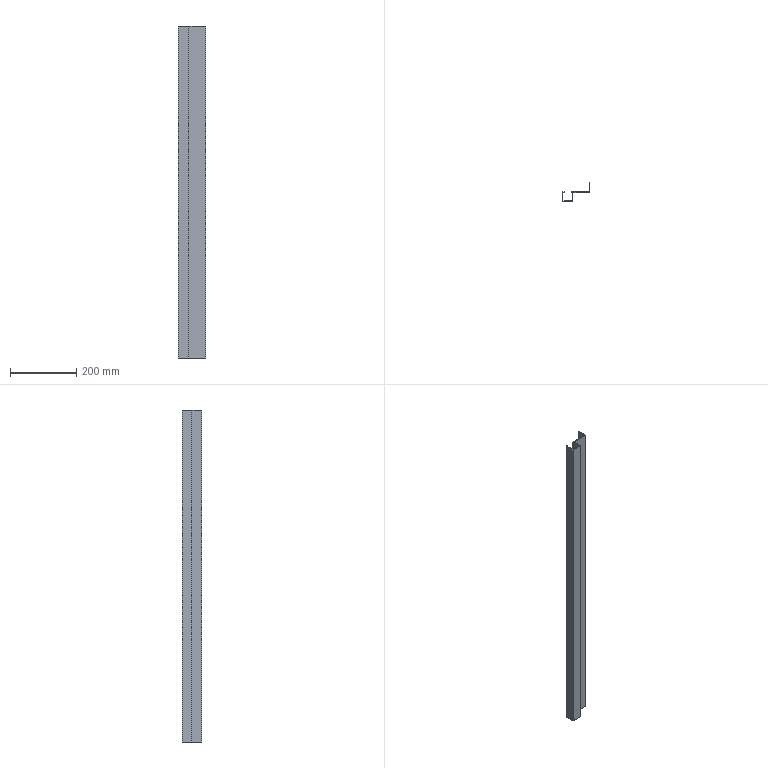Part | STEP file | Rieles_2-22 | 1 solid | 18 faces | box 81.4 x 57.7 x 999 mm | volume 260289 mm3 | plane 18
STEP:
#1=CARTESIAN_POINT('',(10.,26.2,-551.));
#2=VERTEX_POINT('',#1);
#3=CARTESIAN_POINT('',(10.,27.7,-551.));
#4=VERTEX_POINT('',#3);
#5=CARTESIAN_POINT('',(10.,27.35,-551.));
#6=DIRECTION('',(0.,1.,0.));
#7=VECTOR('',#6,1000.);
#8=LINE('',#5,#7);
#9=EDGE_CURVE('',#2,#4,#8,.T.);
#10=ORIENTED_EDGE('',*,*,#9,.T.);
#11=CARTESIAN_POINT('',(64.2,27.7,-551.));
#12=VERTEX_POINT('',#11);
#13=CARTESIAN_POINT('',(25.,27.7,-551.));
#14=DIRECTION('',(1.,0.,0.));
#15=VECTOR('',#14,1000.);
#16=LINE('',#13,#15);
#17=EDGE_CURVE('',#4,#12,#16,.T.);
#18=ORIENTED_EDGE('',*,*,#17,.T.);
#19=CARTESIAN_POINT('',(64.2,56.2,-551.));
#20=VERTEX_POINT('',#19);
#21=CARTESIAN_POINT('',(64.2,27.35,-551.));
#22=DIRECTION('',(0.,1.,0.));
#23=VECTOR('',#22,1000.);
#24=LINE('',#21,#23);
#25=EDGE_CURVE('',#12,#20,#24,.T.);
#26=ORIENTED_EDGE('',*,*,#25,.T.);
#27=CARTESIAN_POINT('',(65.7,56.2,-551.));
#28=VERTEX_POINT('',#27);
#29=CARTESIAN_POINT('',(25.,56.2,-551.));
#30=DIRECTION('',(1.,0.,0.));
#31=VECTOR('',#30,1000.);
#32=LINE('',#29,#31);
#33=EDGE_CURVE('',#20,#28,#32,.T.);
#34=ORIENTED_EDGE('',*,*,#33,.T.);
#35=CARTESIAN_POINT('',(65.7,26.2,-551.));
#36=VERTEX_POINT('',#35);
#37=CARTESIAN_POINT('',(65.7,27.35,-551.));
#38=DIRECTION('',(0.,-1.,0.));
#39=VECTOR('',#38,1000.);
#40=LINE('',#37,#39);
#41=EDGE_CURVE('',#28,#36,#40,.T.);
#42=ORIENTED_EDGE('',*,*,#41,.T.);
#43=CARTESIAN_POINT('',(15.7,26.2,-551.));
#44=VERTEX_POINT('',#43);
#45=CARTESIAN_POINT('',(25.,26.2,-551.));
#46=DIRECTION('',(-1.,0.,0.));
#47=VECTOR('',#46,1000.);
#48=LINE('',#45,#47);
#49=EDGE_CURVE('',#36,#44,#48,.T.);
#50=ORIENTED_EDGE('',*,*,#49,.T.);
#51=CARTESIAN_POINT('',(15.7,-1.5,-551.));
#52=VERTEX_POINT('',#51);
#53=CARTESIAN_POINT('',(15.7,27.35,-551.));
#54=DIRECTION('',(0.,-1.,0.));
#55=VECTOR('',#54,1000.);
#56=LINE('',#53,#55);
#57=EDGE_CURVE('',#44,#52,#56,.T.);
#58=ORIENTED_EDGE('',*,*,#57,.T.);
#59=CARTESIAN_POINT('',(-15.7,-1.5,-551.));
#60=VERTEX_POINT('',#59);
#61=CARTESIAN_POINT('',(25.,-1.5,-551.));
#62=DIRECTION('',(-1.,0.,0.));
#63=VECTOR('',#62,1000.);
#64=LINE('',#61,#63);
#65=EDGE_CURVE('',#52,#60,#64,.T.);
#66=ORIENTED_EDGE('',*,*,#65,.T.);
#67=CARTESIAN_POINT('',(-15.7,27.7,-551.));
#68=VERTEX_POINT('',#67);
#69=CARTESIAN_POINT('',(-15.7,27.35,-551.));
#70=DIRECTION('',(0.,1.,0.));
#71=VECTOR('',#70,1000.);
#72=LINE('',#69,#71);
#73=EDGE_CURVE('',#60,#68,#72,.T.);
#74=ORIENTED_EDGE('',*,*,#73,.T.);
#75=CARTESIAN_POINT('',(-10.,27.7,-551.));
#76=VERTEX_POINT('',#75);
#77=CARTESIAN_POINT('',(25.,27.7,-551.));
#78=DIRECTION('',(1.,0.,0.));
#79=VECTOR('',#78,1000.);
#80=LINE('',#77,#79);
#81=EDGE_CURVE('',#68,#76,#80,.T.);
#82=ORIENTED_EDGE('',*,*,#81,.T.);
#83=CARTESIAN_POINT('',(-10.,26.2,-551.));
#84=VERTEX_POINT('',#83);
#85=CARTESIAN_POINT('',(-10.,27.35,-551.));
#86=DIRECTION('',(0.,-1.,0.));
#87=VECTOR('',#86,1000.);
#88=LINE('',#85,#87);
#89=EDGE_CURVE('',#76,#84,#88,.T.);
#90=ORIENTED_EDGE('',*,*,#89,.T.);
#91=CARTESIAN_POINT('',(-14.2,26.2,-551.));
#92=VERTEX_POINT('',#91);
#93=CARTESIAN_POINT('',(25.,26.2,-551.));
#94=DIRECTION('',(-1.,0.,0.));
#95=VECTOR('',#94,1000.);
#96=LINE('',#93,#95);
#97=EDGE_CURVE('',#84,#92,#96,.T.);
#98=ORIENTED_EDGE('',*,*,#97,.T.);
#99=CARTESIAN_POINT('',(-14.2,0.,-551.));
#100=VERTEX_POINT('',#99);
#101=CARTESIAN_POINT('',(-14.2,27.35,-551.));
#102=DIRECTION('',(0.,-1.,0.));
#103=VECTOR('',#102,1000.);
#104=LINE('',#101,#103);
#105=EDGE_CURVE('',#92,#100,#104,.T.);
#106=ORIENTED_EDGE('',*,*,#105,.T.);
#107=CARTESIAN_POINT('',(14.2,0.,-551.));
#108=VERTEX_POINT('',#107);
#109=CARTESIAN_POINT('',(25.,0.,-551.));
#110=DIRECTION('',(1.,0.,0.));
#111=VECTOR('',#110,1000.);
#112=LINE('',#109,#111);
#113=EDGE_CURVE('',#100,#108,#112,.T.);
#114=ORIENTED_EDGE('',*,*,#113,.T.);
#115=CARTESIAN_POINT('',(14.2,26.2,-551.));
#116=VERTEX_POINT('',#115);
#117=CARTESIAN_POINT('',(14.2,27.35,-551.));
#118=DIRECTION('',(0.,1.,0.));
#119=VECTOR('',#118,1000.);
#120=LINE('',#117,#119);
#121=EDGE_CURVE('',#108,#116,#120,.T.);
#122=ORIENTED_EDGE('',*,*,#121,.T.);
#123=CARTESIAN_POINT('',(25.,26.2,-551.));
#124=DIRECTION('',(-1.,0.,0.));
#125=VECTOR('',#124,1000.);
#126=LINE('',#123,#125);
#127=EDGE_CURVE('',#116,#2,#126,.T.);
#128=ORIENTED_EDGE('',*,*,#127,.T.);
#129=EDGE_LOOP('',(#10,#18,#26,#34,#42,#50,#58,#66,#74,#82,#90,#98,#106,#114,#122,#128));
#130=FACE_OUTER_BOUND('',#129,.T.);
#131=CARTESIAN_POINT('',(25.,27.35,-551.));
#132=DIRECTION('',(0.,0.,-1.));
#133=DIRECTION('',(0.,-1.,0.));
#134=AXIS2_PLACEMENT_3D('',#131,#132,#133);
#135=PLANE('',#134);
#136=ADVANCED_FACE('',(#130),#135,.T.);
#137=CARTESIAN_POINT('',(10.,26.2,448.));
#138=VERTEX_POINT('',#137);
#139=CARTESIAN_POINT('',(10.,27.7,448.));
#140=VERTEX_POINT('',#139);
#141=CARTESIAN_POINT('',(10.,26.2,448.));
#142=DIRECTION('',(0.,1.,0.));
#143=VECTOR('',#142,1000.);
#144=LINE('',#141,#143);
#145=EDGE_CURVE('',#138,#140,#144,.T.);
#146=ORIENTED_EDGE('',*,*,#145,.F.);
#147=CARTESIAN_POINT('',(14.2,26.2,448.));
#148=VERTEX_POINT('',#147);
#149=CARTESIAN_POINT('',(14.2,26.2,448.));
#150=DIRECTION('',(-1.,0.,0.));
#151=VECTOR('',#150,1000.);
#152=LINE('',#149,#151);
#153=EDGE_CURVE('',#148,#138,#152,.T.);
#154=ORIENTED_EDGE('',*,*,#153,.F.);
#155=CARTESIAN_POINT('',(14.2,0.,448.));
#156=VERTEX_POINT('',#155);
#157=CARTESIAN_POINT('',(14.2,0.,448.));
#158=DIRECTION('',(0.,1.,0.));
#159=VECTOR('',#158,1000.);
#160=LINE('',#157,#159);
#161=EDGE_CURVE('',#156,#148,#160,.T.);
#162=ORIENTED_EDGE('',*,*,#161,.F.);
#163=CARTESIAN_POINT('',(-14.2,0.,448.));
#164=VERTEX_POINT('',#163);
#165=CARTESIAN_POINT('',(-14.2,0.,448.));
#166=DIRECTION('',(1.,0.,0.));
#167=VECTOR('',#166,1000.);
#168=LINE('',#165,#167);
#169=EDGE_CURVE('',#164,#156,#168,.T.);
#170=ORIENTED_EDGE('',*,*,#169,.F.);
#171=CARTESIAN_POINT('',(-14.2,26.2,448.));
#172=VERTEX_POINT('',#171);
#173=CARTESIAN_POINT('',(-14.2,26.2,448.));
#174=DIRECTION('',(0.,-1.,0.));
#175=VECTOR('',#174,1000.);
#176=LINE('',#173,#175);
#177=EDGE_CURVE('',#172,#164,#176,.T.);
#178=ORIENTED_EDGE('',*,*,#177,.F.);
#179=CARTESIAN_POINT('',(-10.,26.2,448.));
#180=VERTEX_POINT('',#179);
#181=CARTESIAN_POINT('',(-10.,26.2,448.));
#182=DIRECTION('',(-1.,0.,0.));
#183=VECTOR('',#182,1000.);
#184=LINE('',#181,#183);
#185=EDGE_CURVE('',#180,#172,#184,.T.);
#186=ORIENTED_EDGE('',*,*,#185,.F.);
#187=CARTESIAN_POINT('',(-10.,27.7,448.));
#188=VERTEX_POINT('',#187);
#189=CARTESIAN_POINT('',(-10.,27.7,448.));
#190=DIRECTION('',(0.,-1.,0.));
#191=VECTOR('',#190,1000.);
#192=LINE('',#189,#191);
#193=EDGE_CURVE('',#188,#180,#192,.T.);
#194=ORIENTED_EDGE('',*,*,#193,.F.);
#195=CARTESIAN_POINT('',(-15.7,27.7,448.));
#196=VERTEX_POINT('',#195);
#197=CARTESIAN_POINT('',(-15.7,27.7,448.));
#198=DIRECTION('',(1.,0.,0.));
#199=VECTOR('',#198,1000.);
#200=LINE('',#197,#199);
#201=EDGE_CURVE('',#196,#188,#200,.T.);
#202=ORIENTED_EDGE('',*,*,#201,.F.);
#203=CARTESIAN_POINT('',(-15.7,-1.5,448.));
#204=VERTEX_POINT('',#203);
#205=CARTESIAN_POINT('',(-15.7,-1.5,448.));
#206=DIRECTION('',(0.,1.,0.));
#207=VECTOR('',#206,1000.);
#208=LINE('',#205,#207);
#209=EDGE_CURVE('',#204,#196,#208,.T.);
#210=ORIENTED_EDGE('',*,*,#209,.F.);
#211=CARTESIAN_POINT('',(15.7,-1.5,448.));
#212=VERTEX_POINT('',#211);
#213=CARTESIAN_POINT('',(15.7,-1.5,448.));
#214=DIRECTION('',(-1.,0.,0.));
#215=VECTOR('',#214,1000.);
#216=LINE('',#213,#215);
#217=EDGE_CURVE('',#212,#204,#216,.T.);
#218=ORIENTED_EDGE('',*,*,#217,.F.);
#219=CARTESIAN_POINT('',(15.7,26.2,448.));
#220=VERTEX_POINT('',#219);
#221=CARTESIAN_POINT('',(15.7,26.2,448.));
#222=DIRECTION('',(0.,-1.,0.));
#223=VECTOR('',#222,1000.);
#224=LINE('',#221,#223);
#225=EDGE_CURVE('',#220,#212,#224,.T.);
#226=ORIENTED_EDGE('',*,*,#225,.F.);
#227=CARTESIAN_POINT('',(65.7,26.2,448.));
#228=VERTEX_POINT('',#227);
#229=CARTESIAN_POINT('',(65.7,26.2,448.));
#230=DIRECTION('',(-1.,0.,0.));
#231=VECTOR('',#230,1000.);
#232=LINE('',#229,#231);
#233=EDGE_CURVE('',#228,#220,#232,.T.);
#234=ORIENTED_EDGE('',*,*,#233,.F.);
#235=CARTESIAN_POINT('',(65.7,56.2,448.));
#236=VERTEX_POINT('',#235);
#237=CARTESIAN_POINT('',(65.7,56.2,448.));
#238=DIRECTION('',(0.,-1.,0.));
#239=VECTOR('',#238,1000.);
#240=LINE('',#237,#239);
#241=EDGE_CURVE('',#236,#228,#240,.T.);
#242=ORIENTED_EDGE('',*,*,#241,.F.);
#243=CARTESIAN_POINT('',(64.2,56.2,448.));
#244=VERTEX_POINT('',#243);
#245=CARTESIAN_POINT('',(64.2,56.2,448.));
#246=DIRECTION('',(1.,0.,0.));
#247=VECTOR('',#246,1000.);
#248=LINE('',#245,#247);
#249=EDGE_CURVE('',#244,#236,#248,.T.);
#250=ORIENTED_EDGE('',*,*,#249,.F.);
#251=CARTESIAN_POINT('',(64.2,27.7,448.));
#252=VERTEX_POINT('',#251);
#253=CARTESIAN_POINT('',(64.2,27.7,448.));
#254=DIRECTION('',(0.,1.,0.));
#255=VECTOR('',#254,1000.);
#256=LINE('',#253,#255);
#257=EDGE_CURVE('',#252,#244,#256,.T.);
#258=ORIENTED_EDGE('',*,*,#257,.F.);
#259=CARTESIAN_POINT('',(10.,27.7,448.));
#260=DIRECTION('',(1.,0.,0.));
#261=VECTOR('',#260,1000.);
#262=LINE('',#259,#261);
#263=EDGE_CURVE('',#140,#252,#262,.T.);
#264=ORIENTED_EDGE('',*,*,#263,.F.);
#265=EDGE_LOOP('',(#146,#154,#162,#170,#178,#186,#194,#202,#210,#218,#226,#234,#242,#250,#258,#264));
#266=FACE_OUTER_BOUND('',#265,.T.);
#267=CARTESIAN_POINT('',(25.,27.35,448.));
#268=DIRECTION('',(0.,0.,1.));
#269=DIRECTION('',(1.,0.,0.));
#270=AXIS2_PLACEMENT_3D('',#267,#268,#269);
#271=PLANE('',#270);
#272=ADVANCED_FACE('',(#266),#271,.T.);
#273=ORIENTED_EDGE('',*,*,#145,.T.);
#274=CARTESIAN_POINT('',(10.,27.7,407.));
#275=DIRECTION('',(0.,0.,-1.));
#276=VECTOR('',#275,1000.);
#277=LINE('',#274,#276);
#278=EDGE_CURVE('',#140,#4,#277,.T.);
#279=ORIENTED_EDGE('',*,*,#278,.T.);
#280=ORIENTED_EDGE('',*,*,#9,.F.);
#281=CARTESIAN_POINT('',(10.,26.2,407.));
#282=DIRECTION('',(0.,0.,-1.));
#283=VECTOR('',#282,1000.);
#284=LINE('',#281,#283);
#285=EDGE_CURVE('',#138,#2,#284,.T.);
#286=ORIENTED_EDGE('',*,*,#285,.F.);
#287=EDGE_LOOP('',(#273,#279,#280,#286));
#288=FACE_OUTER_BOUND('',#287,.T.);
#289=CARTESIAN_POINT('',(10.,26.2,407.));
#290=DIRECTION('',(-1.,0.,0.));
#291=DIRECTION('',(0.,0.,1.));
#292=AXIS2_PLACEMENT_3D('',#289,#290,#291);
#293=PLANE('',#292);
#294=ADVANCED_FACE('',(#288),#293,.T.);
#295=ORIENTED_EDGE('',*,*,#263,.T.);
#296=CARTESIAN_POINT('',(64.2,27.7,407.));
#297=DIRECTION('',(0.,0.,-1.));
#298=VECTOR('',#297,1000.);
#299=LINE('',#296,#298);
#300=EDGE_CURVE('',#252,#12,#299,.T.);
#301=ORIENTED_EDGE('',*,*,#300,.T.);
#302=ORIENTED_EDGE('',*,*,#17,.F.);
#303=ORIENTED_EDGE('',*,*,#278,.F.);
#304=EDGE_LOOP('',(#295,#301,#302,#303));
#305=FACE_OUTER_BOUND('',#304,.T.);
#306=CARTESIAN_POINT('',(10.,27.7,407.));
#307=DIRECTION('',(0.,1.,0.));
#308=DIRECTION('',(1.,0.,0.));
#309=AXIS2_PLACEMENT_3D('',#306,#307,#308);
#310=PLANE('',#309);
#311=ADVANCED_FACE('',(#305),#310,.T.);
#312=ORIENTED_EDGE('',*,*,#257,.T.);
#313=CARTESIAN_POINT('',(64.2,56.2,407.));
#314=DIRECTION('',(0.,0.,-1.));
#315=VECTOR('',#314,1000.);
#316=LINE('',#313,#315);
#317=EDGE_CURVE('',#244,#20,#316,.T.);
#318=ORIENTED_EDGE('',*,*,#317,.T.);
#319=ORIENTED_EDGE('',*,*,#25,.F.);
#320=ORIENTED_EDGE('',*,*,#300,.F.);
#321=EDGE_LOOP('',(#312,#318,#319,#320));
#322=FACE_OUTER_BOUND('',#321,.T.);
#323=CARTESIAN_POINT('',(64.2,27.7,407.));
#324=DIRECTION('',(-1.,0.,0.));
#325=DIRECTION('',(0.,0.,1.));
#326=AXIS2_PLACEMENT_3D('',#323,#324,#325);
#327=PLANE('',#326);
#328=ADVANCED_FACE('',(#322),#327,.T.);
#329=ORIENTED_EDGE('',*,*,#249,.T.);
#330=CARTESIAN_POINT('',(65.7,56.2,407.));
#331=DIRECTION('',(0.,0.,-1.));
#332=VECTOR('',#331,1000.);
#333=LINE('',#330,#332);
#334=EDGE_CURVE('',#236,#28,#333,.T.);
#335=ORIENTED_EDGE('',*,*,#334,.T.);
#336=ORIENTED_EDGE('',*,*,#33,.F.);
#337=ORIENTED_EDGE('',*,*,#317,.F.);
#338=EDGE_LOOP('',(#329,#335,#336,#337));
#339=FACE_OUTER_BOUND('',#338,.T.);
#340=CARTESIAN_POINT('',(64.2,56.2,407.));
#341=DIRECTION('',(0.,1.,0.));
#342=DIRECTION('',(1.,0.,0.));
#343=AXIS2_PLACEMENT_3D('',#340,#341,#342);
#344=PLANE('',#343);
#345=ADVANCED_FACE('',(#339),#344,.T.);
#346=ORIENTED_EDGE('',*,*,#241,.T.);
#347=CARTESIAN_POINT('',(65.7,26.2,407.));
#348=DIRECTION('',(0.,0.,-1.));
#349=VECTOR('',#348,1000.);
#350=LINE('',#347,#349);
#351=EDGE_CURVE('',#228,#36,#350,.T.);
#352=ORIENTED_EDGE('',*,*,#351,.T.);
#353=ORIENTED_EDGE('',*,*,#41,.F.);
#354=ORIENTED_EDGE('',*,*,#334,.F.);
#355=EDGE_LOOP('',(#346,#352,#353,#354));
#356=FACE_OUTER_BOUND('',#355,.T.);
#357=CARTESIAN_POINT('',(65.7,56.2,407.));
#358=DIRECTION('',(1.,0.,0.));
#359=DIRECTION('',(0.,-1.,0.));
#360=AXIS2_PLACEMENT_3D('',#357,#358,#359);
#361=PLANE('',#360);
#362=ADVANCED_FACE('',(#356),#361,.T.);
#363=ORIENTED_EDGE('',*,*,#233,.T.);
#364=CARTESIAN_POINT('',(15.7,26.2,407.));
#365=DIRECTION('',(0.,0.,-1.));
#366=VECTOR('',#365,1000.);
#367=LINE('',#364,#366);
#368=EDGE_CURVE('',#220,#44,#367,.T.);
#369=ORIENTED_EDGE('',*,*,#368,.T.);
#370=ORIENTED_EDGE('',*,*,#49,.F.);
#371=ORIENTED_EDGE('',*,*,#351,.F.);
#372=EDGE_LOOP('',(#363,#369,#370,#371));
#373=FACE_OUTER_BOUND('',#372,.T.);
#374=CARTESIAN_POINT('',(65.7,26.2,407.));
#375=DIRECTION('',(0.,-1.,0.));
#376=DIRECTION('',(0.,0.,-1.));
#377=AXIS2_PLACEMENT_3D('',#374,#375,#376);
#378=PLANE('',#377);
#379=ADVANCED_FACE('',(#373),#378,.T.);
#380=ORIENTED_EDGE('',*,*,#225,.T.);
#381=CARTESIAN_POINT('',(15.7,-1.5,407.));
#382=DIRECTION('',(0.,0.,-1.));
#383=VECTOR('',#382,1000.);
#384=LINE('',#381,#383);
#385=EDGE_CURVE('',#212,#52,#384,.T.);
#386=ORIENTED_EDGE('',*,*,#385,.T.);
#387=ORIENTED_EDGE('',*,*,#57,.F.);
#388=ORIENTED_EDGE('',*,*,#368,.F.);
#389=EDGE_LOOP('',(#380,#386,#387,#388));
#390=FACE_OUTER_BOUND('',#389,.T.);
#391=CARTESIAN_POINT('',(15.7,26.2,407.));
#392=DIRECTION('',(1.,0.,0.));
#393=DIRECTION('',(0.,1.,0.));
#394=AXIS2_PLACEMENT_3D('',#391,#392,#393);
#395=PLANE('',#394);
#396=ADVANCED_FACE('',(#390),#395,.T.);
#397=ORIENTED_EDGE('',*,*,#217,.T.);
#398=CARTESIAN_POINT('',(-15.7,-1.5,407.));
#399=DIRECTION('',(0.,0.,-1.));
#400=VECTOR('',#399,1000.);
#401=LINE('',#398,#400);
#402=EDGE_CURVE('',#204,#60,#401,.T.);
#403=ORIENTED_EDGE('',*,*,#402,.T.);
#404=ORIENTED_EDGE('',*,*,#65,.F.);
#405=ORIENTED_EDGE('',*,*,#385,.F.);
#406=EDGE_LOOP('',(#397,#403,#404,#405));
#407=FACE_OUTER_BOUND('',#406,.T.);
#408=CARTESIAN_POINT('',(15.7,-1.5,407.));
#409=DIRECTION('',(0.,-1.,0.));
#410=DIRECTION('',(0.,0.,-1.));
#411=AXIS2_PLACEMENT_3D('',#408,#409,#410);
#412=PLANE('',#411);
#413=ADVANCED_FACE('',(#407),#412,.T.);
#414=ORIENTED_EDGE('',*,*,#209,.T.);
#415=CARTESIAN_POINT('',(-15.7,27.7,407.));
#416=DIRECTION('',(0.,0.,-1.));
#417=VECTOR('',#416,1000.);
#418=LINE('',#415,#417);
#419=EDGE_CURVE('',#196,#68,#418,.T.);
#420=ORIENTED_EDGE('',*,*,#419,.T.);
#421=ORIENTED_EDGE('',*,*,#73,.F.);
#422=ORIENTED_EDGE('',*,*,#402,.F.);
#423=EDGE_LOOP('',(#414,#420,#421,#422));
#424=FACE_OUTER_BOUND('',#423,.T.);
#425=CARTESIAN_POINT('',(-15.7,-1.5,407.));
#426=DIRECTION('',(-1.,0.,0.));
#427=DIRECTION('',(0.,0.,1.));
#428=AXIS2_PLACEMENT_3D('',#425,#426,#427);
#429=PLANE('',#428);
#430=ADVANCED_FACE('',(#424),#429,.T.);
#431=ORIENTED_EDGE('',*,*,#201,.T.);
#432=CARTESIAN_POINT('',(-10.,27.7,407.));
#433=DIRECTION('',(0.,0.,-1.));
#434=VECTOR('',#433,1000.);
#435=LINE('',#432,#434);
#436=EDGE_CURVE('',#188,#76,#435,.T.);
#437=ORIENTED_EDGE('',*,*,#436,.T.);
#438=ORIENTED_EDGE('',*,*,#81,.F.);
#439=ORIENTED_EDGE('',*,*,#419,.F.);
#440=EDGE_LOOP('',(#431,#437,#438,#439));
#441=FACE_OUTER_BOUND('',#440,.T.);
#442=CARTESIAN_POINT('',(-15.7,27.7,407.));
#443=DIRECTION('',(0.,1.,0.));
#444=DIRECTION('',(1.,0.,0.));
#445=AXIS2_PLACEMENT_3D('',#442,#443,#444);
#446=PLANE('',#445);
#447=ADVANCED_FACE('',(#441),#446,.T.);
#448=ORIENTED_EDGE('',*,*,#193,.T.);
#449=CARTESIAN_POINT('',(-10.,26.2,407.));
#450=DIRECTION('',(0.,0.,-1.));
#451=VECTOR('',#450,1000.);
#452=LINE('',#449,#451);
#453=EDGE_CURVE('',#180,#84,#452,.T.);
#454=ORIENTED_EDGE('',*,*,#453,.T.);
#455=ORIENTED_EDGE('',*,*,#89,.F.);
#456=ORIENTED_EDGE('',*,*,#436,.F.);
#457=EDGE_LOOP('',(#448,#454,#455,#456));
#458=FACE_OUTER_BOUND('',#457,.T.);
#459=CARTESIAN_POINT('',(-10.,27.7,407.));
#460=DIRECTION('',(1.,0.,0.));
#461=DIRECTION('',(0.,1.,0.));
#462=AXIS2_PLACEMENT_3D('',#459,#460,#461);
#463=PLANE('',#462);
#464=ADVANCED_FACE('',(#458),#463,.T.);
#465=ORIENTED_EDGE('',*,*,#185,.T.);
#466=CARTESIAN_POINT('',(-14.2,26.2,407.));
#467=DIRECTION('',(0.,0.,-1.));
#468=VECTOR('',#467,1000.);
#469=LINE('',#466,#468);
#470=EDGE_CURVE('',#172,#92,#469,.T.);
#471=ORIENTED_EDGE('',*,*,#470,.T.);
#472=ORIENTED_EDGE('',*,*,#97,.F.);
#473=ORIENTED_EDGE('',*,*,#453,.F.);
#474=EDGE_LOOP('',(#465,#471,#472,#473));
#475=FACE_OUTER_BOUND('',#474,.T.);
#476=CARTESIAN_POINT('',(-10.,26.2,407.));
#477=DIRECTION('',(0.,-1.,0.));
#478=DIRECTION('',(0.,0.,-1.));
#479=AXIS2_PLACEMENT_3D('',#476,#477,#478);
#480=PLANE('',#479);
#481=ADVANCED_FACE('',(#475),#480,.T.);
#482=ORIENTED_EDGE('',*,*,#177,.T.);
#483=CARTESIAN_POINT('',(-14.2,0.,407.));
#484=DIRECTION('',(0.,0.,-1.));
#485=VECTOR('',#484,1000.);
#486=LINE('',#483,#485);
#487=EDGE_CURVE('',#164,#100,#486,.T.);
#488=ORIENTED_EDGE('',*,*,#487,.T.);
#489=ORIENTED_EDGE('',*,*,#105,.F.);
#490=ORIENTED_EDGE('',*,*,#470,.F.);
#491=EDGE_LOOP('',(#482,#488,#489,#490));
#492=FACE_OUTER_BOUND('',#491,.T.);
#493=CARTESIAN_POINT('',(-14.2,26.2,407.));
#494=DIRECTION('',(1.,0.,0.));
#495=DIRECTION('',(0.,1.,0.));
#496=AXIS2_PLACEMENT_3D('',#493,#494,#495);
#497=PLANE('',#496);
#498=ADVANCED_FACE('',(#492),#497,.T.);
#499=ORIENTED_EDGE('',*,*,#169,.T.);
#500=CARTESIAN_POINT('',(14.2,0.,407.));
#501=DIRECTION('',(0.,0.,-1.));
#502=VECTOR('',#501,1000.);
#503=LINE('',#500,#502);
#504=EDGE_CURVE('',#156,#108,#503,.T.);
#505=ORIENTED_EDGE('',*,*,#504,.T.);
#506=ORIENTED_EDGE('',*,*,#113,.F.);
#507=ORIENTED_EDGE('',*,*,#487,.F.);
#508=EDGE_LOOP('',(#499,#505,#506,#507));
#509=FACE_OUTER_BOUND('',#508,.T.);
#510=CARTESIAN_POINT('',(-14.2,0.,407.));
#511=DIRECTION('',(0.,1.,0.));
#512=DIRECTION('',(1.,0.,0.));
#513=AXIS2_PLACEMENT_3D('',#510,#511,#512);
#514=PLANE('',#513);
#515=ADVANCED_FACE('',(#509),#514,.T.);
#516=ORIENTED_EDGE('',*,*,#161,.T.);
#517=CARTESIAN_POINT('',(14.2,26.2,407.));
#518=DIRECTION('',(0.,0.,-1.));
#519=VECTOR('',#518,1000.);
#520=LINE('',#517,#519);
#521=EDGE_CURVE('',#148,#116,#520,.T.);
#522=ORIENTED_EDGE('',*,*,#521,.T.);
#523=ORIENTED_EDGE('',*,*,#121,.F.);
#524=ORIENTED_EDGE('',*,*,#504,.F.);
#525=EDGE_LOOP('',(#516,#522,#523,#524));
#526=FACE_OUTER_BOUND('',#525,.T.);
#527=CARTESIAN_POINT('',(14.2,0.,407.));
#528=DIRECTION('',(-1.,0.,0.));
#529=DIRECTION('',(0.,0.,1.));
#530=AXIS2_PLACEMENT_3D('',#527,#528,#529);
#531=PLANE('',#530);
#532=ADVANCED_FACE('',(#526),#531,.T.);
#533=ORIENTED_EDGE('',*,*,#153,.T.);
#534=ORIENTED_EDGE('',*,*,#285,.T.);
#535=ORIENTED_EDGE('',*,*,#127,.F.);
#536=ORIENTED_EDGE('',*,*,#521,.F.);
#537=EDGE_LOOP('',(#533,#534,#535,#536));
#538=FACE_OUTER_BOUND('',#537,.T.);
#539=CARTESIAN_POINT('',(14.2,26.2,407.));
#540=DIRECTION('',(0.,-1.,0.));
#541=DIRECTION('',(-1.,0.,0.));
#542=AXIS2_PLACEMENT_3D('',#539,#540,#541);
#543=PLANE('',#542);
#544=ADVANCED_FACE('',(#538),#543,.T.);
#545=CLOSED_SHELL('',(#136,#272,#294,#311,#328,#345,#362,#379,#396,#413,#430,#447,#464,#481,#498,#515,#532,#544));
#546=MANIFOLD_SOLID_BREP('',#545);
#547=CARTESIAN_POINT('',(0.,0.,0.));
#548=DIRECTION('',(0.,0.,1.));
#549=DIRECTION('',(1.,0.,0.));
#550=AXIS2_PLACEMENT_3D('',#547,#548,#549);
#551=(LENGTH_UNIT()NAMED_UNIT(*)SI_UNIT(.MILLI.,.METRE.));
#552=UNCERTAINTY_MEASURE_WITH_UNIT(LENGTH_MEASURE(0.00001),#551,'','');
#553=(NAMED_UNIT(*)PLANE_ANGLE_UNIT()SI_UNIT($,.RADIAN.));
#554=(NAMED_UNIT(*)SI_UNIT($,.STERADIAN.)SOLID_ANGLE_UNIT());
#555=(GEOMETRIC_REPRESENTATION_CONTEXT(3)GLOBAL_UNCERTAINTY_ASSIGNED_CONTEXT((#552))GLOBAL_UNIT_ASSIGNED_CONTEXT((#551,#553,#554))REPRESENTATION_CONTEXT('',''));
#556=ADVANCED_BREP_SHAPE_REPRESENTATION('',(#546,#550),#555);